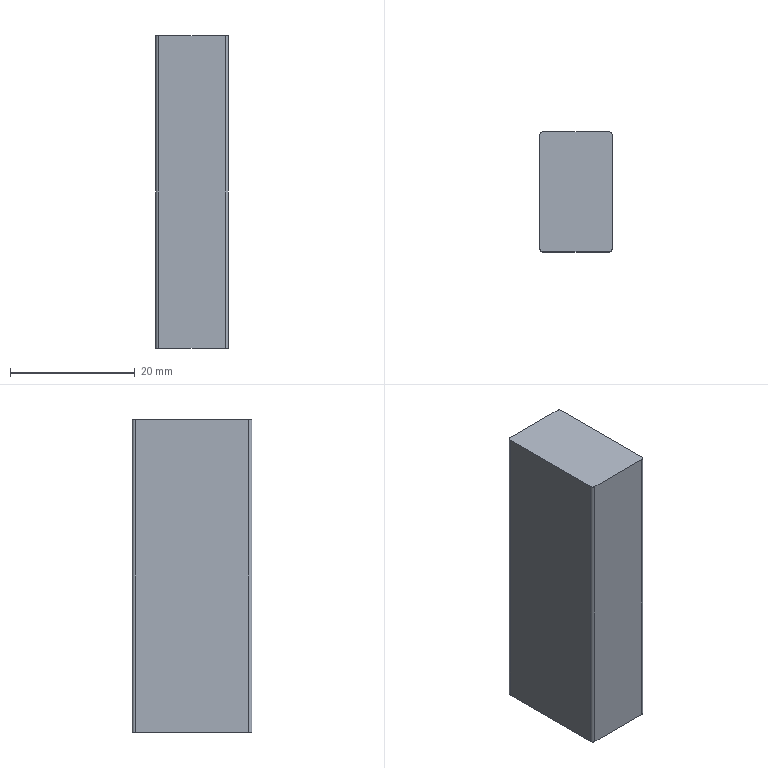Part | NX | features BREP 1 | 1 solid | 10 faces | box 11.615 x 19.2 x 50 mm | volume 11140 mm3 | plane 6 | cylinder 4 | commonest cylinder face diameters 1 x4
STEP:
#1=CARTESIAN_POINT('',(-5.308,9.6,-40.6));
#2=VERTEX_POINT('',#1);
#3=CARTESIAN_POINT('',(-5.808,9.1,-40.6));
#4=VERTEX_POINT('',#3);
#5=CARTESIAN_POINT('',(-5.308,9.1,-40.6));
#6=DIRECTION('',(0.,0.,1.));
#7=DIRECTION('',(1.,0.,0.));
#8=AXIS2_PLACEMENT_3D('',#5,#6,#7);
#9=CIRCLE('',#8,0.5);
#10=EDGE_CURVE('',#2,#4,#9,.T.);
#11=ORIENTED_EDGE('',*,*,#10,.F.);
#12=CARTESIAN_POINT('',(-5.308,9.6,-90.6));
#13=VERTEX_POINT('',#12);
#14=CARTESIAN_POINT('',(-5.308,9.6,-90.6));
#15=DIRECTION('',(0.,0.,1.));
#16=VECTOR('',#15,1000.);
#17=LINE('',#14,#16);
#18=EDGE_CURVE('',#13,#2,#17,.T.);
#19=ORIENTED_EDGE('',*,*,#18,.F.);
#20=CARTESIAN_POINT('',(-5.808,9.1,-90.6));
#21=VERTEX_POINT('',#20);
#22=CARTESIAN_POINT('',(-5.308,9.1,-90.6));
#23=DIRECTION('',(0.,0.,1.));
#24=DIRECTION('',(1.,0.,0.));
#25=AXIS2_PLACEMENT_3D('',#22,#23,#24);
#26=CIRCLE('',#25,0.5);
#27=EDGE_CURVE('',#13,#21,#26,.T.);
#28=ORIENTED_EDGE('',*,*,#27,.T.);
#29=CARTESIAN_POINT('',(-5.808,9.1,-90.6));
#30=DIRECTION('',(0.,0.,1.));
#31=VECTOR('',#30,1000.);
#32=LINE('',#29,#31);
#33=EDGE_CURVE('',#21,#4,#32,.T.);
#34=ORIENTED_EDGE('',*,*,#33,.T.);
#35=EDGE_LOOP('',(#11,#19,#28,#34));
#36=FACE_BOUND('',#35,.T.);
#37=CARTESIAN_POINT('',(-5.308,9.1,-90.6));
#38=DIRECTION('',(0.,0.,1.));
#39=DIRECTION('',(-1.,0.,0.));
#40=AXIS2_PLACEMENT_3D('',#37,#38,#39);
#41=CYLINDRICAL_SURFACE('',#40,0.5);
#42=ADVANCED_FACE('',(#36),#41,.T.);
#43=CARTESIAN_POINT('',(-5.808,-9.1,-40.6));
#44=VERTEX_POINT('',#43);
#45=CARTESIAN_POINT('',(-5.808,-9.1,-40.6));
#46=DIRECTION('',(0.,1.,0.));
#47=VECTOR('',#46,1000.);
#48=LINE('',#45,#47);
#49=EDGE_CURVE('',#44,#4,#48,.T.);
#50=ORIENTED_EDGE('',*,*,#49,.T.);
#51=ORIENTED_EDGE('',*,*,#33,.F.);
#52=CARTESIAN_POINT('',(-5.808,-9.1,-90.6));
#53=VERTEX_POINT('',#52);
#54=CARTESIAN_POINT('',(-5.808,-9.1,-90.6));
#55=DIRECTION('',(0.,1.,0.));
#56=VECTOR('',#55,1000.);
#57=LINE('',#54,#56);
#58=EDGE_CURVE('',#53,#21,#57,.T.);
#59=ORIENTED_EDGE('',*,*,#58,.F.);
#60=CARTESIAN_POINT('',(-5.808,-9.1,-90.6));
#61=DIRECTION('',(0.,0.,1.));
#62=VECTOR('',#61,1000.);
#63=LINE('',#60,#62);
#64=EDGE_CURVE('',#53,#44,#63,.T.);
#65=ORIENTED_EDGE('',*,*,#64,.T.);
#66=EDGE_LOOP('',(#50,#51,#59,#65));
#67=FACE_BOUND('',#66,.T.);
#68=CARTESIAN_POINT('',(-5.808,-9.1,-90.6));
#69=DIRECTION('',(1.,0.,0.));
#70=DIRECTION('',(0.,-1.,0.));
#71=AXIS2_PLACEMENT_3D('',#68,#69,#70);
#72=PLANE('',#71);
#73=ADVANCED_FACE('',(#67),#72,.F.);
#74=CARTESIAN_POINT('',(-5.308,-9.6,-40.6));
#75=VERTEX_POINT('',#74);
#76=CARTESIAN_POINT('',(-5.308,-9.1,-40.6));
#77=DIRECTION('',(0.,0.,1.));
#78=DIRECTION('',(1.,0.,0.));
#79=AXIS2_PLACEMENT_3D('',#76,#77,#78);
#80=CIRCLE('',#79,0.5);
#81=EDGE_CURVE('',#44,#75,#80,.T.);
#82=ORIENTED_EDGE('',*,*,#81,.F.);
#83=ORIENTED_EDGE('',*,*,#64,.F.);
#84=CARTESIAN_POINT('',(-5.308,-9.6,-90.6));
#85=VERTEX_POINT('',#84);
#86=CARTESIAN_POINT('',(-5.308,-9.1,-90.6));
#87=DIRECTION('',(0.,0.,1.));
#88=DIRECTION('',(1.,0.,0.));
#89=AXIS2_PLACEMENT_3D('',#86,#87,#88);
#90=CIRCLE('',#89,0.5);
#91=EDGE_CURVE('',#53,#85,#90,.T.);
#92=ORIENTED_EDGE('',*,*,#91,.T.);
#93=CARTESIAN_POINT('',(-5.308,-9.6,-90.6));
#94=DIRECTION('',(0.,0.,1.));
#95=VECTOR('',#94,1000.);
#96=LINE('',#93,#95);
#97=EDGE_CURVE('',#85,#75,#96,.T.);
#98=ORIENTED_EDGE('',*,*,#97,.T.);
#99=EDGE_LOOP('',(#82,#83,#92,#98));
#100=FACE_BOUND('',#99,.T.);
#101=CARTESIAN_POINT('',(-5.308,-9.1,-90.6));
#102=DIRECTION('',(0.,0.,1.));
#103=DIRECTION('',(-1.,0.,0.));
#104=AXIS2_PLACEMENT_3D('',#101,#102,#103);
#105=CYLINDRICAL_SURFACE('',#104,0.5);
#106=ADVANCED_FACE('',(#100),#105,.T.);
#107=CARTESIAN_POINT('',(5.308,-9.6,-40.6));
#108=VERTEX_POINT('',#107);
#109=CARTESIAN_POINT('',(5.308,-9.6,-40.6));
#110=DIRECTION('',(-1.,0.,0.));
#111=VECTOR('',#110,1000.);
#112=LINE('',#109,#111);
#113=EDGE_CURVE('',#108,#75,#112,.T.);
#114=ORIENTED_EDGE('',*,*,#113,.T.);
#115=ORIENTED_EDGE('',*,*,#97,.F.);
#116=CARTESIAN_POINT('',(5.308,-9.6,-90.6));
#117=VERTEX_POINT('',#116);
#118=CARTESIAN_POINT('',(5.308,-9.6,-90.6));
#119=DIRECTION('',(-1.,0.,0.));
#120=VECTOR('',#119,1000.);
#121=LINE('',#118,#120);
#122=EDGE_CURVE('',#117,#85,#121,.T.);
#123=ORIENTED_EDGE('',*,*,#122,.F.);
#124=CARTESIAN_POINT('',(5.308,-9.6,-90.6));
#125=DIRECTION('',(0.,0.,1.));
#126=VECTOR('',#125,1000.);
#127=LINE('',#124,#126);
#128=EDGE_CURVE('',#117,#108,#127,.T.);
#129=ORIENTED_EDGE('',*,*,#128,.T.);
#130=EDGE_LOOP('',(#114,#115,#123,#129));
#131=FACE_BOUND('',#130,.T.);
#132=CARTESIAN_POINT('',(5.308,-9.6,-90.6));
#133=DIRECTION('',(0.,1.,0.));
#134=DIRECTION('',(0.,0.,-1.));
#135=AXIS2_PLACEMENT_3D('',#132,#133,#134);
#136=PLANE('',#135);
#137=ADVANCED_FACE('',(#131),#136,.F.);
#138=CARTESIAN_POINT('',(5.808,-9.1,-40.6));
#139=VERTEX_POINT('',#138);
#140=CARTESIAN_POINT('',(5.308,-9.1,-40.6));
#141=DIRECTION('',(0.,0.,1.));
#142=DIRECTION('',(1.,0.,0.));
#143=AXIS2_PLACEMENT_3D('',#140,#141,#142);
#144=CIRCLE('',#143,0.5);
#145=EDGE_CURVE('',#108,#139,#144,.T.);
#146=ORIENTED_EDGE('',*,*,#145,.F.);
#147=ORIENTED_EDGE('',*,*,#128,.F.);
#148=CARTESIAN_POINT('',(5.808,-9.1,-90.6));
#149=VERTEX_POINT('',#148);
#150=CARTESIAN_POINT('',(5.308,-9.1,-90.6));
#151=DIRECTION('',(0.,0.,1.));
#152=DIRECTION('',(1.,0.,0.));
#153=AXIS2_PLACEMENT_3D('',#150,#151,#152);
#154=CIRCLE('',#153,0.5);
#155=EDGE_CURVE('',#117,#149,#154,.T.);
#156=ORIENTED_EDGE('',*,*,#155,.T.);
#157=CARTESIAN_POINT('',(5.808,-9.1,-90.6));
#158=DIRECTION('',(0.,0.,1.));
#159=VECTOR('',#158,1000.);
#160=LINE('',#157,#159);
#161=EDGE_CURVE('',#149,#139,#160,.T.);
#162=ORIENTED_EDGE('',*,*,#161,.T.);
#163=EDGE_LOOP('',(#146,#147,#156,#162));
#164=FACE_BOUND('',#163,.T.);
#165=CARTESIAN_POINT('',(5.308,-9.1,-90.6));
#166=DIRECTION('',(0.,0.,1.));
#167=DIRECTION('',(-1.,0.,0.));
#168=AXIS2_PLACEMENT_3D('',#165,#166,#167);
#169=CYLINDRICAL_SURFACE('',#168,0.5);
#170=ADVANCED_FACE('',(#164),#169,.T.);
#171=CARTESIAN_POINT('',(5.808,9.1,-40.6));
#172=VERTEX_POINT('',#171);
#173=CARTESIAN_POINT('',(5.808,9.1,-40.6));
#174=DIRECTION('',(0.,-1.,0.));
#175=VECTOR('',#174,1000.);
#176=LINE('',#173,#175);
#177=EDGE_CURVE('',#172,#139,#176,.T.);
#178=ORIENTED_EDGE('',*,*,#177,.T.);
#179=ORIENTED_EDGE('',*,*,#161,.F.);
#180=CARTESIAN_POINT('',(5.808,9.1,-90.6));
#181=VERTEX_POINT('',#180);
#182=CARTESIAN_POINT('',(5.808,9.1,-90.6));
#183=DIRECTION('',(0.,-1.,0.));
#184=VECTOR('',#183,1000.);
#185=LINE('',#182,#184);
#186=EDGE_CURVE('',#181,#149,#185,.T.);
#187=ORIENTED_EDGE('',*,*,#186,.F.);
#188=CARTESIAN_POINT('',(5.808,9.1,-90.6));
#189=DIRECTION('',(0.,0.,1.));
#190=VECTOR('',#189,1000.);
#191=LINE('',#188,#190);
#192=EDGE_CURVE('',#181,#172,#191,.T.);
#193=ORIENTED_EDGE('',*,*,#192,.T.);
#194=EDGE_LOOP('',(#178,#179,#187,#193));
#195=FACE_BOUND('',#194,.T.);
#196=CARTESIAN_POINT('',(5.808,9.1,-90.6));
#197=DIRECTION('',(-1.,0.,0.));
#198=DIRECTION('',(0.,0.,-1.));
#199=AXIS2_PLACEMENT_3D('',#196,#197,#198);
#200=PLANE('',#199);
#201=ADVANCED_FACE('',(#195),#200,.F.);
#202=CARTESIAN_POINT('',(5.308,9.6,-40.6));
#203=VERTEX_POINT('',#202);
#204=CARTESIAN_POINT('',(5.308,9.1,-40.6));
#205=DIRECTION('',(0.,0.,1.));
#206=DIRECTION('',(1.,0.,0.));
#207=AXIS2_PLACEMENT_3D('',#204,#205,#206);
#208=CIRCLE('',#207,0.5);
#209=EDGE_CURVE('',#172,#203,#208,.T.);
#210=ORIENTED_EDGE('',*,*,#209,.F.);
#211=ORIENTED_EDGE('',*,*,#192,.F.);
#212=CARTESIAN_POINT('',(5.308,9.6,-90.6));
#213=VERTEX_POINT('',#212);
#214=CARTESIAN_POINT('',(5.308,9.1,-90.6));
#215=DIRECTION('',(0.,0.,1.));
#216=DIRECTION('',(1.,0.,0.));
#217=AXIS2_PLACEMENT_3D('',#214,#215,#216);
#218=CIRCLE('',#217,0.5);
#219=EDGE_CURVE('',#181,#213,#218,.T.);
#220=ORIENTED_EDGE('',*,*,#219,.T.);
#221=CARTESIAN_POINT('',(5.308,9.6,-90.6));
#222=DIRECTION('',(0.,0.,1.));
#223=VECTOR('',#222,1000.);
#224=LINE('',#221,#223);
#225=EDGE_CURVE('',#213,#203,#224,.T.);
#226=ORIENTED_EDGE('',*,*,#225,.T.);
#227=EDGE_LOOP('',(#210,#211,#220,#226));
#228=FACE_BOUND('',#227,.T.);
#229=CARTESIAN_POINT('',(5.308,9.1,-90.6));
#230=DIRECTION('',(0.,0.,1.));
#231=DIRECTION('',(-1.,0.,0.));
#232=AXIS2_PLACEMENT_3D('',#229,#230,#231);
#233=CYLINDRICAL_SURFACE('',#232,0.5);
#234=ADVANCED_FACE('',(#228),#233,.T.);
#235=CARTESIAN_POINT('',(-5.308,9.6,-40.6));
#236=DIRECTION('',(1.,0.,0.));
#237=VECTOR('',#236,1000.);
#238=LINE('',#235,#237);
#239=EDGE_CURVE('',#2,#203,#238,.T.);
#240=ORIENTED_EDGE('',*,*,#239,.T.);
#241=ORIENTED_EDGE('',*,*,#225,.F.);
#242=CARTESIAN_POINT('',(-5.308,9.6,-90.6));
#243=DIRECTION('',(1.,0.,0.));
#244=VECTOR('',#243,1000.);
#245=LINE('',#242,#244);
#246=EDGE_CURVE('',#13,#213,#245,.T.);
#247=ORIENTED_EDGE('',*,*,#246,.F.);
#248=ORIENTED_EDGE('',*,*,#18,.T.);
#249=EDGE_LOOP('',(#240,#241,#247,#248));
#250=FACE_BOUND('',#249,.T.);
#251=CARTESIAN_POINT('',(-5.308,9.6,-90.6));
#252=DIRECTION('',(0.,-1.,0.));
#253=DIRECTION('',(-1.,0.,0.));
#254=AXIS2_PLACEMENT_3D('',#251,#252,#253);
#255=PLANE('',#254);
#256=ADVANCED_FACE('',(#250),#255,.F.);
#257=ORIENTED_EDGE('',*,*,#27,.F.);
#258=ORIENTED_EDGE('',*,*,#246,.T.);
#259=ORIENTED_EDGE('',*,*,#219,.F.);
#260=ORIENTED_EDGE('',*,*,#186,.T.);
#261=ORIENTED_EDGE('',*,*,#155,.F.);
#262=ORIENTED_EDGE('',*,*,#122,.T.);
#263=ORIENTED_EDGE('',*,*,#91,.F.);
#264=ORIENTED_EDGE('',*,*,#58,.T.);
#265=EDGE_LOOP('',(#257,#258,#259,#260,#261,#262,#263,#264));
#266=FACE_BOUND('',#265,.T.);
#267=CARTESIAN_POINT('',(-5.308,9.1,-90.6));
#268=DIRECTION('',(0.,0.,1.));
#269=DIRECTION('',(-1.,0.,0.));
#270=AXIS2_PLACEMENT_3D('',#267,#268,#269);
#271=PLANE('',#270);
#272=ADVANCED_FACE('',(#266),#271,.F.);
#273=ORIENTED_EDGE('',*,*,#10,.T.);
#274=ORIENTED_EDGE('',*,*,#49,.F.);
#275=ORIENTED_EDGE('',*,*,#81,.T.);
#276=ORIENTED_EDGE('',*,*,#113,.F.);
#277=ORIENTED_EDGE('',*,*,#145,.T.);
#278=ORIENTED_EDGE('',*,*,#177,.F.);
#279=ORIENTED_EDGE('',*,*,#209,.T.);
#280=ORIENTED_EDGE('',*,*,#239,.F.);
#281=EDGE_LOOP('',(#273,#274,#275,#276,#277,#278,#279,#280));
#282=FACE_BOUND('',#281,.T.);
#283=CARTESIAN_POINT('',(-5.308,9.1,-40.6));
#284=DIRECTION('',(0.,0.,1.));
#285=DIRECTION('',(-1.,0.,0.));
#286=AXIS2_PLACEMENT_3D('',#283,#284,#285);
#287=PLANE('',#286);
#288=ADVANCED_FACE('',(#282),#287,.T.);
#289=CLOSED_SHELL('',(#42,#73,#106,#137,#170,#201,#234,#256,#272,#288));
#290=MANIFOLD_SOLID_BREP('',#289);
#291=(LENGTH_UNIT()NAMED_UNIT(*)SI_UNIT(.MILLI.,.METRE.));
#292=UNCERTAINTY_MEASURE_WITH_UNIT(LENGTH_MEASURE(0.00001),#291,'','');
#293=(NAMED_UNIT(*)PLANE_ANGLE_UNIT()SI_UNIT($,.RADIAN.));
#294=(NAMED_UNIT(*)SI_UNIT($,.STERADIAN.)SOLID_ANGLE_UNIT());
#295=(GEOMETRIC_REPRESENTATION_CONTEXT(3)GLOBAL_UNCERTAINTY_ASSIGNED_CONTEXT((#292))GLOBAL_UNIT_ASSIGNED_CONTEXT((#291,#293,#294))REPRESENTATION_CONTEXT('',''));
#296=ADVANCED_BREP_SHAPE_REPRESENTATION('',(#290),#295);